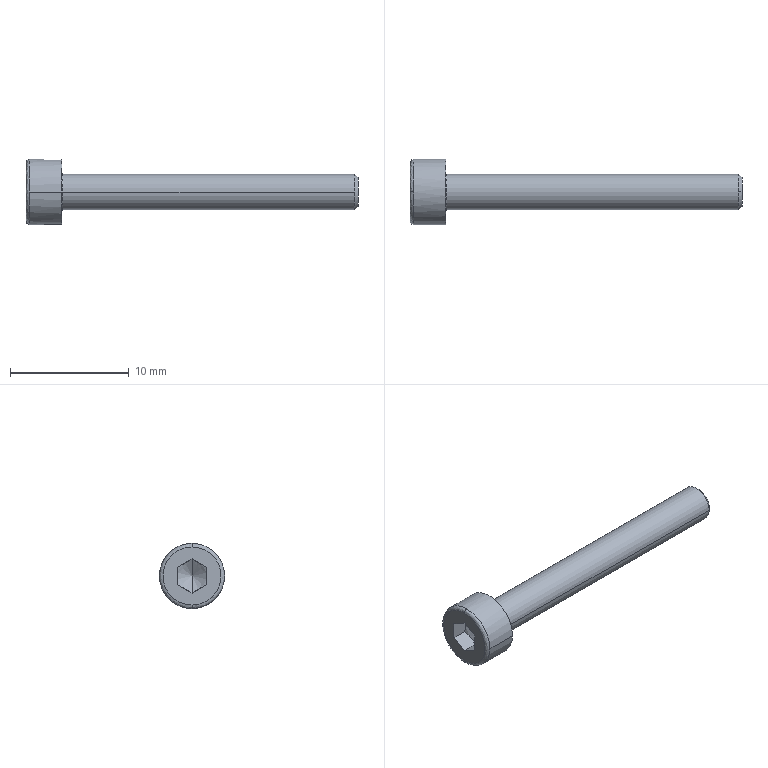Part | STEP file | 0217_304_SCB3-25 | 1 solid | 21 faces | box 28 x 5.5 x 5.5 mm | volume 238.258 mm3 | plane 9 | cylinder 4 | cone 4 | spline 2 | torus 2 | commonest cylinder face diameters 3 x2 5.5 x2